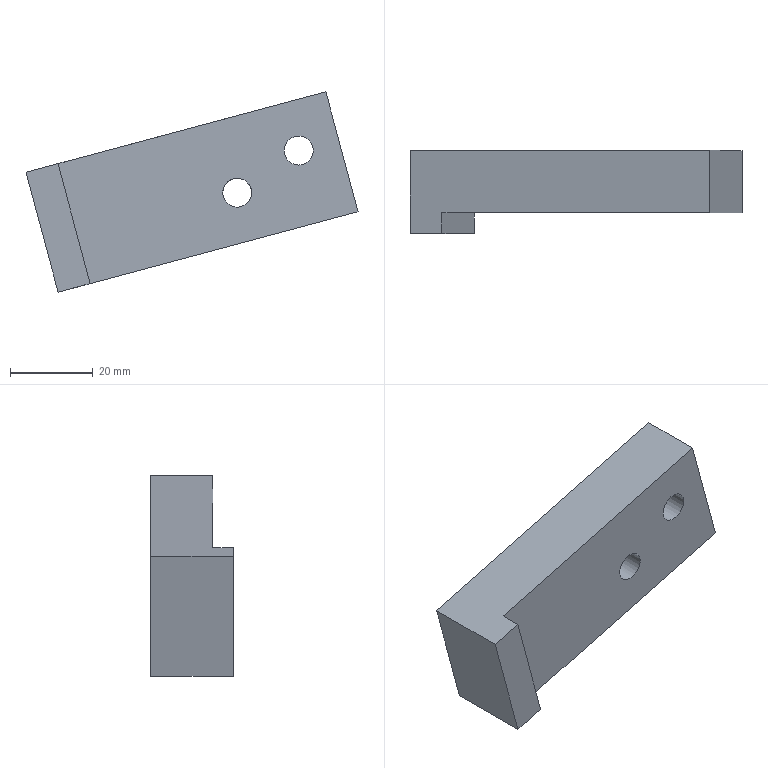Part | NX | features solid 2 | 1 solid | 14 faces | box 80.209 x 20 x 48.389 mm | volume 32774 mm3 | plane 10 | cylinder 4 | commonest cylinder face diameters 7.007 x2 11.008 x2
STEP:
#1=CARTESIAN_POINT('',(916.048,89.937,-24.569));
#2=VERTEX_POINT('',#1);
#3=CARTESIAN_POINT('',(843.603,89.937,-43.98));
#4=VERTEX_POINT('',#3);
#5=CARTESIAN_POINT('',(901.559,89.937,-28.451));
#6=DIRECTION('',(0.9659,-0.000000134,0.2588));
#7=VECTOR('',#6,1000.);
#8=LINE('',#5,#7);
#9=EDGE_CURVE('',#2,#4,#8,.F.);
#10=ORIENTED_EDGE('',*,*,#9,.T.);
#11=CARTESIAN_POINT('',(835.839,89.937,-15.002));
#12=VERTEX_POINT('',#11);
#13=CARTESIAN_POINT('',(853.956,89.937,-82.617));
#14=DIRECTION('',(-0.2588,-0.000000499,0.9659));
#15=VECTOR('',#14,1000.);
#16=LINE('',#13,#15);
#17=EDGE_CURVE('',#4,#12,#16,.T.);
#18=ORIENTED_EDGE('',*,*,#17,.T.);
#19=CARTESIAN_POINT('',(908.283,89.937,4.409));
#20=VERTEX_POINT('',#19);
#21=CARTESIAN_POINT('',(893.794,89.937,0.5267));
#22=DIRECTION('',(0.9659,-0.000000134,0.2588));
#23=VECTOR('',#22,1000.);
#24=LINE('',#21,#23);
#25=EDGE_CURVE('',#20,#12,#24,.F.);
#26=ORIENTED_EDGE('',*,*,#25,.F.);
#27=CARTESIAN_POINT('',(926.401,89.937,-63.206));
#28=DIRECTION('',(-0.2588,-0.000000499,0.9659));
#29=VECTOR('',#28,1000.);
#30=LINE('',#27,#29);
#31=EDGE_CURVE('',#2,#20,#30,.T.);
#32=ORIENTED_EDGE('',*,*,#31,.F.);
#33=EDGE_LOOP('',(#10,#18,#26,#32));
#34=FACE_BOUND('',#33,.T.);
#35=CARTESIAN_POINT('',(882.095,89.937,-22.718));
#36=VERTEX_POINT('',#35);
#37=CARTESIAN_POINT('',(886.862,89.937,-19.966));
#38=DIRECTION('',(0.,1.,0.000000517));
#39=DIRECTION('',(-0.866,0.000000258,-0.5));
#40=AXIS2_PLACEMENT_3D('',#37,#38,#39);
#41=CIRCLE('',#40,5.504);
#42=EDGE_CURVE('',#36,#36,#41,.T.);
#43=ORIENTED_EDGE('',*,*,#42,.F.);
#44=EDGE_LOOP('',(#43));
#45=FACE_BOUND('',#44,.T.);
#46=CARTESIAN_POINT('',(896.226,89.937,-9.77));
#47=VERTEX_POINT('',#46);
#48=CARTESIAN_POINT('',(901.73,89.937,-9.77));
#49=DIRECTION('',(0.,-1.,-0.000000517));
#50=DIRECTION('',(-1.,0.,0.));
#51=AXIS2_PLACEMENT_3D('',#48,#49,#50);
#52=CIRCLE('',#51,5.504);
#53=EDGE_CURVE('',#47,#47,#52,.T.);
#54=ORIENTED_EDGE('',*,*,#53,.T.);
#55=EDGE_LOOP('',(#54));
#56=FACE_BOUND('',#55,.T.);
#57=CARTESIAN_POINT('',(911.912,89.937,-67.088));
#58=DIRECTION('',(0.,1.,0.000000517));
#59=DIRECTION('',(-0.2588,-0.000000499,0.9659));
#60=AXIS2_PLACEMENT_3D('',#57,#58,#59);
#61=PLANE('',#60);
#62=ADVANCED_FACE('',(#34,#45,#56),#61,.T.);
#63=CARTESIAN_POINT('',(916.048,74.937,-24.569));
#64=VERTEX_POINT('',#63);
#65=CARTESIAN_POINT('',(851.331,74.937,-41.91));
#66=VERTEX_POINT('',#65);
#67=CARTESIAN_POINT('',(901.559,74.937,-28.451));
#68=DIRECTION('',(-0.9659,0.000000134,-0.2588));
#69=VECTOR('',#68,1000.);
#70=LINE('',#67,#69);
#71=EDGE_CURVE('',#64,#66,#70,.T.);
#72=ORIENTED_EDGE('',*,*,#71,.T.);
#73=CARTESIAN_POINT('',(851.331,69.937,-41.91));
#74=VERTEX_POINT('',#73);
#75=CARTESIAN_POINT('',(851.331,74.937,-41.91));
#76=DIRECTION('',(0.,1.,0.000000517));
#77=VECTOR('',#76,1000.);
#78=LINE('',#75,#77);
#79=EDGE_CURVE('',#66,#74,#78,.F.);
#80=ORIENTED_EDGE('',*,*,#79,.T.);
#81=CARTESIAN_POINT('',(843.603,69.937,-43.98));
#82=VERTEX_POINT('',#81);
#83=CARTESIAN_POINT('',(901.559,69.937,-28.451));
#84=DIRECTION('',(-0.9659,0.000000134,-0.2588));
#85=VECTOR('',#84,1000.);
#86=LINE('',#83,#85);
#87=EDGE_CURVE('',#74,#82,#86,.T.);
#88=ORIENTED_EDGE('',*,*,#87,.T.);
#89=CARTESIAN_POINT('',(843.603,74.937,-43.98));
#90=DIRECTION('',(0.,1.,0.000000517));
#91=VECTOR('',#90,1000.);
#92=LINE('',#89,#91);
#93=EDGE_CURVE('',#82,#4,#92,.T.);
#94=ORIENTED_EDGE('',*,*,#93,.T.);
#95=ORIENTED_EDGE('',*,*,#9,.F.);
#96=CARTESIAN_POINT('',(916.048,74.937,-24.569));
#97=DIRECTION('',(0.,1.,0.000000517));
#98=VECTOR('',#97,1000.);
#99=LINE('',#96,#98);
#100=EDGE_CURVE('',#64,#2,#99,.T.);
#101=ORIENTED_EDGE('',*,*,#100,.F.);
#102=EDGE_LOOP('',(#72,#80,#88,#94,#95,#101));
#103=FACE_BOUND('',#102,.T.);
#104=CARTESIAN_POINT('',(901.559,74.937,-28.451));
#105=DIRECTION('',(0.2588,0.000000499,-0.9659));
#106=DIRECTION('',(-0.9659,0.000000134,-0.2588));
#107=AXIS2_PLACEMENT_3D('',#104,#105,#106);
#108=PLANE('',#107);
#109=ADVANCED_FACE('',(#103),#108,.T.);
#110=ORIENTED_EDGE('',*,*,#25,.T.);
#111=CARTESIAN_POINT('',(835.839,69.937,-15.002));
#112=VERTEX_POINT('',#111);
#113=CARTESIAN_POINT('',(835.839,74.937,-15.002));
#114=DIRECTION('',(0.,1.,0.000000517));
#115=VECTOR('',#114,1000.);
#116=LINE('',#113,#115);
#117=EDGE_CURVE('',#112,#12,#116,.T.);
#118=ORIENTED_EDGE('',*,*,#117,.F.);
#119=CARTESIAN_POINT('',(843.566,69.937,-12.932));
#120=VERTEX_POINT('',#119);
#121=CARTESIAN_POINT('',(893.794,69.937,0.5267));
#122=DIRECTION('',(0.9659,-0.000000134,0.2588));
#123=VECTOR('',#122,1000.);
#124=LINE('',#121,#123);
#125=EDGE_CURVE('',#120,#112,#124,.F.);
#126=ORIENTED_EDGE('',*,*,#125,.F.);
#127=CARTESIAN_POINT('',(843.566,74.937,-12.932));
#128=VERTEX_POINT('',#127);
#129=CARTESIAN_POINT('',(843.566,74.937,-12.932));
#130=DIRECTION('',(0.,1.,0.000000517));
#131=VECTOR('',#130,1000.);
#132=LINE('',#129,#131);
#133=EDGE_CURVE('',#128,#120,#132,.F.);
#134=ORIENTED_EDGE('',*,*,#133,.F.);
#135=CARTESIAN_POINT('',(908.283,74.937,4.409));
#136=VERTEX_POINT('',#135);
#137=CARTESIAN_POINT('',(893.794,74.937,0.5267));
#138=DIRECTION('',(-0.9659,0.000000134,-0.2588));
#139=VECTOR('',#138,1000.);
#140=LINE('',#137,#139);
#141=EDGE_CURVE('',#136,#128,#140,.T.);
#142=ORIENTED_EDGE('',*,*,#141,.F.);
#143=CARTESIAN_POINT('',(908.283,74.937,4.409));
#144=DIRECTION('',(0.,1.,0.000000517));
#145=VECTOR('',#144,1000.);
#146=LINE('',#143,#145);
#147=EDGE_CURVE('',#136,#20,#146,.T.);
#148=ORIENTED_EDGE('',*,*,#147,.T.);
#149=EDGE_LOOP('',(#110,#118,#126,#134,#142,#148));
#150=FACE_BOUND('',#149,.T.);
#151=CARTESIAN_POINT('',(893.794,74.937,0.5267));
#152=DIRECTION('',(0.2588,0.000000499,-0.9659));
#153=DIRECTION('',(-0.9659,0.000000134,-0.2588));
#154=AXIS2_PLACEMENT_3D('',#151,#152,#153);
#155=PLANE('',#154);
#156=ADVANCED_FACE('',(#150),#155,.F.);
#157=CARTESIAN_POINT('',(901.73,74.937,-13.274));
#158=VERTEX_POINT('',#157);
#159=CARTESIAN_POINT('',(901.73,74.937,-9.77));
#160=DIRECTION('',(0.,1.,0.000000517));
#161=DIRECTION('',(0.,0.000000517,-1.));
#162=AXIS2_PLACEMENT_3D('',#159,#160,#161);
#163=CIRCLE('',#162,3.503);
#164=EDGE_CURVE('',#158,#158,#163,.T.);
#165=ORIENTED_EDGE('',*,*,#164,.T.);
#166=EDGE_LOOP('',(#165));
#167=FACE_BOUND('',#166,.T.);
#168=CARTESIAN_POINT('',(886.862,74.937,-23.469));
#169=VERTEX_POINT('',#168);
#170=CARTESIAN_POINT('',(886.862,74.937,-19.966));
#171=DIRECTION('',(0.,1.,0.000000517));
#172=DIRECTION('',(0.,0.000000517,-1.));
#173=AXIS2_PLACEMENT_3D('',#170,#171,#172);
#174=CIRCLE('',#173,3.503);
#175=EDGE_CURVE('',#169,#169,#174,.T.);
#176=ORIENTED_EDGE('',*,*,#175,.T.);
#177=EDGE_LOOP('',(#176));
#178=FACE_BOUND('',#177,.T.);
#179=CARTESIAN_POINT('',(861.684,74.937,-80.547));
#180=DIRECTION('',(-0.2588,-0.000000499,0.9659));
#181=VECTOR('',#180,1000.);
#182=LINE('',#179,#181);
#183=EDGE_CURVE('',#66,#128,#182,.T.);
#184=ORIENTED_EDGE('',*,*,#183,.F.);
#185=ORIENTED_EDGE('',*,*,#71,.F.);
#186=CARTESIAN_POINT('',(1073.831,74.937,-613.424));
#187=DIRECTION('',(-0.2588,-0.000000499,0.9659));
#188=VECTOR('',#187,1000.);
#189=LINE('',#186,#188);
#190=EDGE_CURVE('',#64,#136,#189,.T.);
#191=ORIENTED_EDGE('',*,*,#190,.T.);
#192=ORIENTED_EDGE('',*,*,#141,.T.);
#193=EDGE_LOOP('',(#184,#185,#191,#192));
#194=FACE_BOUND('',#193,.T.);
#195=CARTESIAN_POINT('',(911.912,74.937,-67.088));
#196=DIRECTION('',(0.,1.,0.000000517));
#197=DIRECTION('',(-0.2588,-0.000000499,0.9659));
#198=AXIS2_PLACEMENT_3D('',#195,#196,#197);
#199=PLANE('',#198);
#200=ADVANCED_FACE('',(#167,#178,#194),#199,.F.);
#201=ORIENTED_EDGE('',*,*,#190,.F.);
#202=ORIENTED_EDGE('',*,*,#100,.T.);
#203=ORIENTED_EDGE('',*,*,#31,.T.);
#204=ORIENTED_EDGE('',*,*,#147,.F.);
#205=EDGE_LOOP('',(#201,#202,#203,#204));
#206=FACE_BOUND('',#205,.T.);
#207=CARTESIAN_POINT('',(1073.831,74.937,-613.424));
#208=DIRECTION('',(-0.9659,0.000000134,-0.2588));
#209=DIRECTION('',(-0.2588,-0.000000499,0.9659));
#210=AXIS2_PLACEMENT_3D('',#207,#208,#209);
#211=PLANE('',#210);
#212=ADVANCED_FACE('',(#206),#211,.F.);
#213=ORIENTED_EDGE('',*,*,#79,.F.);
#214=ORIENTED_EDGE('',*,*,#183,.T.);
#215=ORIENTED_EDGE('',*,*,#133,.T.);
#216=CARTESIAN_POINT('',(847.449,69.937,-27.421));
#217=DIRECTION('',(0.2588,0.000000499,-0.9659));
#218=VECTOR('',#217,1000.);
#219=LINE('',#216,#218);
#220=EDGE_CURVE('',#120,#74,#219,.T.);
#221=ORIENTED_EDGE('',*,*,#220,.T.);
#222=EDGE_LOOP('',(#213,#214,#215,#221));
#223=FACE_BOUND('',#222,.T.);
#224=CARTESIAN_POINT('',(847.449,84.937,-27.421));
#225=DIRECTION('',(-0.9659,0.000000134,-0.2588));
#226=DIRECTION('',(0.2588,0.,-0.9659));
#227=AXIS2_PLACEMENT_3D('',#224,#225,#226);
#228=PLANE('',#227);
#229=ADVANCED_FACE('',(#223),#228,.F.);
#230=ORIENTED_EDGE('',*,*,#93,.F.);
#231=CARTESIAN_POINT('',(853.956,69.937,-82.617));
#232=DIRECTION('',(-0.2588,-0.000000499,0.9659));
#233=VECTOR('',#232,1000.);
#234=LINE('',#231,#233);
#235=EDGE_CURVE('',#82,#112,#234,.T.);
#236=ORIENTED_EDGE('',*,*,#235,.T.);
#237=ORIENTED_EDGE('',*,*,#117,.T.);
#238=ORIENTED_EDGE('',*,*,#17,.F.);
#239=EDGE_LOOP('',(#230,#236,#237,#238));
#240=FACE_BOUND('',#239,.T.);
#241=CARTESIAN_POINT('',(853.956,74.937,-82.617));
#242=DIRECTION('',(-0.9659,0.000000134,-0.2588));
#243=DIRECTION('',(-0.2588,-0.000000499,0.9659));
#244=AXIS2_PLACEMENT_3D('',#241,#242,#243);
#245=PLANE('',#244);
#246=ADVANCED_FACE('',(#240),#245,.T.);
#247=ORIENTED_EDGE('',*,*,#87,.F.);
#248=ORIENTED_EDGE('',*,*,#220,.F.);
#249=ORIENTED_EDGE('',*,*,#125,.T.);
#250=ORIENTED_EDGE('',*,*,#235,.F.);
#251=EDGE_LOOP('',(#247,#248,#249,#250));
#252=FACE_BOUND('',#251,.T.);
#253=CARTESIAN_POINT('',(911.912,69.937,-67.088));
#254=DIRECTION('',(0.,1.,0.000000517));
#255=DIRECTION('',(-0.2588,-0.000000499,0.9659));
#256=AXIS2_PLACEMENT_3D('',#253,#254,#255);
#257=PLANE('',#256);
#258=ADVANCED_FACE('',(#252),#257,.F.);
#259=CARTESIAN_POINT('',(888.614,80.937,-23.));
#260=VERTEX_POINT('',#259);
#261=CARTESIAN_POINT('',(886.862,80.937,-19.966));
#262=DIRECTION('',(0.,1.,0.000000517));
#263=DIRECTION('',(0.5,0.000000448,-0.866));
#264=AXIS2_PLACEMENT_3D('',#261,#262,#263);
#265=CIRCLE('',#264,3.503);
#266=EDGE_CURVE('',#260,#260,#265,.T.);
#267=ORIENTED_EDGE('',*,*,#266,.T.);
#268=EDGE_LOOP('',(#267));
#269=FACE_BOUND('',#268,.T.);
#270=ORIENTED_EDGE('',*,*,#175,.F.);
#271=EDGE_LOOP('',(#270));
#272=FACE_BOUND('',#271,.T.);
#273=CARTESIAN_POINT('',(886.862,89.937,-19.966));
#274=DIRECTION('',(0.,-1.,-0.000000517));
#275=DIRECTION('',(-0.866,0.000000258,-0.5));
#276=AXIS2_PLACEMENT_3D('',#273,#274,#275);
#277=CYLINDRICAL_SURFACE('',#276,3.503);
#278=ADVANCED_FACE('',(#269,#272),#277,.F.);
#279=ORIENTED_EDGE('',*,*,#266,.F.);
#280=EDGE_LOOP('',(#279));
#281=FACE_BOUND('',#280,.T.);
#282=CARTESIAN_POINT('',(882.095,80.937,-22.718));
#283=VERTEX_POINT('',#282);
#284=CARTESIAN_POINT('',(886.862,80.937,-19.966));
#285=DIRECTION('',(0.,-1.,-0.000000517));
#286=DIRECTION('',(-0.866,0.000000258,-0.5));
#287=AXIS2_PLACEMENT_3D('',#284,#285,#286);
#288=CIRCLE('',#287,5.504);
#289=EDGE_CURVE('',#283,#283,#288,.F.);
#290=ORIENTED_EDGE('',*,*,#289,.T.);
#291=EDGE_LOOP('',(#290));
#292=FACE_BOUND('',#291,.T.);
#293=CARTESIAN_POINT('',(886.862,80.937,-19.966));
#294=DIRECTION('',(0.,-1.,-0.000000517));
#295=DIRECTION('',(0.5,0.000000448,-0.866));
#296=AXIS2_PLACEMENT_3D('',#293,#294,#295);
#297=PLANE('',#296);
#298=ADVANCED_FACE('',(#281,#292),#297,.F.);
#299=ORIENTED_EDGE('',*,*,#289,.F.);
#300=EDGE_LOOP('',(#299));
#301=FACE_BOUND('',#300,.T.);
#302=ORIENTED_EDGE('',*,*,#42,.T.);
#303=EDGE_LOOP('',(#302));
#304=FACE_BOUND('',#303,.T.);
#305=CARTESIAN_POINT('',(886.862,89.937,-19.966));
#306=DIRECTION('',(0.,-1.,-0.000000517));
#307=DIRECTION('',(-0.866,0.000000258,-0.5));
#308=AXIS2_PLACEMENT_3D('',#305,#306,#307);
#309=CYLINDRICAL_SURFACE('',#308,5.504);
#310=ADVANCED_FACE('',(#301,#304),#309,.F.);
#311=CARTESIAN_POINT('',(901.73,80.937,-6.267));
#312=VERTEX_POINT('',#311);
#313=CARTESIAN_POINT('',(901.73,80.937,-9.77));
#314=DIRECTION('',(0.,-1.,-0.000000517));
#315=DIRECTION('',(0.,-0.000000517,1.));
#316=AXIS2_PLACEMENT_3D('',#313,#314,#315);
#317=CIRCLE('',#316,3.503);
#318=EDGE_CURVE('',#312,#312,#317,.T.);
#319=ORIENTED_EDGE('',*,*,#318,.F.);
#320=EDGE_LOOP('',(#319));
#321=FACE_BOUND('',#320,.T.);
#322=ORIENTED_EDGE('',*,*,#164,.F.);
#323=EDGE_LOOP('',(#322));
#324=FACE_BOUND('',#323,.T.);
#325=CARTESIAN_POINT('',(901.73,89.937,-9.77));
#326=DIRECTION('',(0.,-1.,-0.000000517));
#327=DIRECTION('',(-1.,0.,0.));
#328=AXIS2_PLACEMENT_3D('',#325,#326,#327);
#329=CYLINDRICAL_SURFACE('',#328,3.503);
#330=ADVANCED_FACE('',(#321,#324),#329,.F.);
#331=ORIENTED_EDGE('',*,*,#318,.T.);
#332=EDGE_LOOP('',(#331));
#333=FACE_BOUND('',#332,.T.);
#334=CARTESIAN_POINT('',(896.226,80.937,-9.77));
#335=VERTEX_POINT('',#334);
#336=CARTESIAN_POINT('',(901.73,80.937,-9.77));
#337=DIRECTION('',(0.,1.,0.000000517));
#338=DIRECTION('',(-1.,0.,0.));
#339=AXIS2_PLACEMENT_3D('',#336,#337,#338);
#340=CIRCLE('',#339,5.504);
#341=EDGE_CURVE('',#335,#335,#340,.F.);
#342=ORIENTED_EDGE('',*,*,#341,.F.);
#343=EDGE_LOOP('',(#342));
#344=FACE_BOUND('',#343,.T.);
#345=CARTESIAN_POINT('',(901.73,80.937,-9.77));
#346=DIRECTION('',(0.,-1.,-0.000000517));
#347=DIRECTION('',(0.,-0.000000517,1.));
#348=AXIS2_PLACEMENT_3D('',#345,#346,#347);
#349=PLANE('',#348);
#350=ADVANCED_FACE('',(#333,#344),#349,.F.);
#351=ORIENTED_EDGE('',*,*,#341,.T.);
#352=EDGE_LOOP('',(#351));
#353=FACE_BOUND('',#352,.T.);
#354=ORIENTED_EDGE('',*,*,#53,.F.);
#355=EDGE_LOOP('',(#354));
#356=FACE_BOUND('',#355,.T.);
#357=CARTESIAN_POINT('',(901.73,89.937,-9.77));
#358=DIRECTION('',(0.,-1.,-0.000000517));
#359=DIRECTION('',(-1.,0.,0.));
#360=AXIS2_PLACEMENT_3D('',#357,#358,#359);
#361=CYLINDRICAL_SURFACE('',#360,5.504);
#362=ADVANCED_FACE('',(#353,#356),#361,.F.);
#363=CLOSED_SHELL('',(#62,#109,#156,#200,#212,#229,#246,#258,#278,#298,#310,#330,#350,#362));
#364=MANIFOLD_SOLID_BREP('',#363);
#365=(LENGTH_UNIT()NAMED_UNIT(*)SI_UNIT(.MILLI.,.METRE.));
#366=UNCERTAINTY_MEASURE_WITH_UNIT(LENGTH_MEASURE(0.00001),#365,'','');
#367=(NAMED_UNIT(*)PLANE_ANGLE_UNIT()SI_UNIT($,.RADIAN.));
#368=(NAMED_UNIT(*)SI_UNIT($,.STERADIAN.)SOLID_ANGLE_UNIT());
#369=(GEOMETRIC_REPRESENTATION_CONTEXT(3)GLOBAL_UNCERTAINTY_ASSIGNED_CONTEXT((#366))GLOBAL_UNIT_ASSIGNED_CONTEXT((#365,#367,#368))REPRESENTATION_CONTEXT('',''));
#370=ADVANCED_BREP_SHAPE_REPRESENTATION('',(#364),#369);